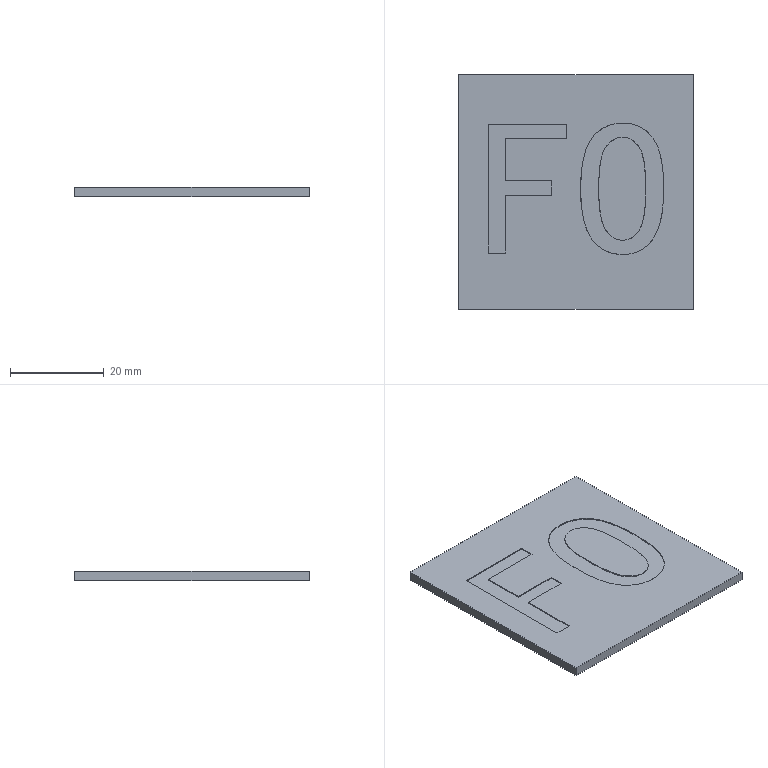Part | STEP file | lll_id1630_x_t | 1 solid | 22 faces | box 50 x 50 x 2 mm | volume 4919 mm3 | plane 19 | other 3
STEP:
#1=CARTESIAN_POINT('',(2722.277,-531.694,3.259));
#2=VERTEX_POINT('',#1);
#3=CARTESIAN_POINT('',(2739.088,-531.694,3.259));
#4=VERTEX_POINT('',#3);
#5=CARTESIAN_POINT('',(2730.683,-531.694,3.259));
#6=DIRECTION('',(1.,0.,0.));
#7=VECTOR('',#6,1.);
#8=LINE('',#5,#7);
#9=EDGE_CURVE('',#2,#4,#8,.T.);
#10=ORIENTED_EDGE('',*,*,#9,.T.);
#11=CARTESIAN_POINT('',(2739.088,-534.734,3.259));
#12=VERTEX_POINT('',#11);
#13=CARTESIAN_POINT('',(2739.088,-533.214,3.259));
#14=DIRECTION('',(0.,-1.,0.));
#15=VECTOR('',#14,1.);
#16=LINE('',#13,#15);
#17=EDGE_CURVE('',#4,#12,#16,.T.);
#18=ORIENTED_EDGE('',*,*,#17,.T.);
#19=CARTESIAN_POINT('',(2725.962,-534.734,3.259));
#20=VERTEX_POINT('',#19);
#21=CARTESIAN_POINT('',(2732.525,-534.734,3.259));
#22=DIRECTION('',(-1.,0.,0.));
#23=VECTOR('',#22,1.);
#24=LINE('',#21,#23);
#25=EDGE_CURVE('',#12,#20,#24,.T.);
#26=ORIENTED_EDGE('',*,*,#25,.T.);
#27=CARTESIAN_POINT('',(2725.962,-543.702,3.259));
#28=VERTEX_POINT('',#27);
#29=CARTESIAN_POINT('',(2725.962,-539.218,3.259));
#30=DIRECTION('',(0.,-1.,0.));
#31=VECTOR('',#30,1.);
#32=LINE('',#29,#31);
#33=EDGE_CURVE('',#20,#28,#32,.T.);
#34=ORIENTED_EDGE('',*,*,#33,.T.);
#35=CARTESIAN_POINT('',(2735.884,-543.702,3.259));
#36=VERTEX_POINT('',#35);
#37=CARTESIAN_POINT('',(2730.923,-543.702,3.259));
#38=DIRECTION('',(1.,0.,0.));
#39=VECTOR('',#38,1.);
#40=LINE('',#37,#39);
#41=EDGE_CURVE('',#28,#36,#40,.T.);
#42=ORIENTED_EDGE('',*,*,#41,.T.);
#43=CARTESIAN_POINT('',(2735.884,-546.742,3.259));
#44=VERTEX_POINT('',#43);
#45=CARTESIAN_POINT('',(2735.884,-545.222,3.259));
#46=DIRECTION('',(0.,-1.,0.));
#47=VECTOR('',#46,1.);
#48=LINE('',#45,#47);
#49=EDGE_CURVE('',#36,#44,#48,.T.);
#50=ORIENTED_EDGE('',*,*,#49,.T.);
#51=CARTESIAN_POINT('',(2725.962,-546.742,3.259));
#52=VERTEX_POINT('',#51);
#53=CARTESIAN_POINT('',(2730.923,-546.742,3.259));
#54=DIRECTION('',(-1.,0.,0.));
#55=VECTOR('',#54,1.);
#56=LINE('',#53,#55);
#57=EDGE_CURVE('',#44,#52,#56,.T.);
#58=ORIENTED_EDGE('',*,*,#57,.T.);
#59=CARTESIAN_POINT('',(2725.962,-559.065,3.259));
#60=VERTEX_POINT('',#59);
#61=CARTESIAN_POINT('',(2725.962,-552.903,3.259));
#62=DIRECTION('',(0.,-1.,0.));
#63=VECTOR('',#62,1.);
#64=LINE('',#61,#63);
#65=EDGE_CURVE('',#52,#60,#64,.T.);
#66=ORIENTED_EDGE('',*,*,#65,.T.);
#67=CARTESIAN_POINT('',(2722.277,-559.065,3.259));
#68=VERTEX_POINT('',#67);
#69=CARTESIAN_POINT('',(2724.119,-559.065,3.259));
#70=DIRECTION('',(-1.,0.,0.));
#71=VECTOR('',#70,1.);
#72=LINE('',#69,#71);
#73=EDGE_CURVE('',#60,#68,#72,.T.);
#74=ORIENTED_EDGE('',*,*,#73,.T.);
#75=CARTESIAN_POINT('',(2722.277,-545.38,3.259));
#76=DIRECTION('',(0.,1.,0.));
#77=VECTOR('',#76,1.);
#78=LINE('',#75,#77);
#79=EDGE_CURVE('',#68,#2,#78,.T.);
#80=ORIENTED_EDGE('',*,*,#79,.T.);
#81=EDGE_LOOP('',(#10,#18,#26,#34,#42,#50,#58,#66,#74,#80));
#82=FACE_BOUND('',#81,.T.);
#83=CARTESIAN_POINT('',(2766.009,-571.065,3.259));
#84=VERTEX_POINT('',#83);
#85=CARTESIAN_POINT('',(2716.009,-571.065,3.259));
#86=VERTEX_POINT('',#85);
#87=CARTESIAN_POINT('',(2816.009,-571.065,3.259));
#88=DIRECTION('',(-1.,0.,0.));
#89=VECTOR('',#88,1.);
#90=LINE('',#87,#89);
#91=EDGE_CURVE('',#84,#86,#90,.T.);
#92=ORIENTED_EDGE('',*,*,#91,.F.);
#93=CARTESIAN_POINT('',(2766.009,-521.065,3.259));
#94=VERTEX_POINT('',#93);
#95=CARTESIAN_POINT('',(2766.009,-471.065,3.259));
#96=DIRECTION('',(0.,-1.,0.));
#97=VECTOR('',#96,1.);
#98=LINE('',#95,#97);
#99=EDGE_CURVE('',#94,#84,#98,.T.);
#100=ORIENTED_EDGE('',*,*,#99,.F.);
#101=CARTESIAN_POINT('',(2716.009,-521.065,3.259));
#102=VERTEX_POINT('',#101);
#103=CARTESIAN_POINT('',(2816.009,-521.065,3.259));
#104=DIRECTION('',(-1.,0.,0.));
#105=VECTOR('',#104,1.);
#106=LINE('',#103,#105);
#107=EDGE_CURVE('',#94,#102,#106,.T.);
#108=ORIENTED_EDGE('',*,*,#107,.T.);
#109=CARTESIAN_POINT('',(2716.009,-471.065,3.259));
#110=DIRECTION('',(0.,1.,0.));
#111=VECTOR('',#110,1.);
#112=LINE('',#109,#111);
#113=EDGE_CURVE('',#86,#102,#112,.T.);
#114=ORIENTED_EDGE('',*,*,#113,.F.);
#115=EDGE_LOOP('',(#92,#100,#108,#114));
#116=FACE_BOUND('',#115,.T.);
#117=CARTESIAN_POINT('',(2744.372,-556.108,3.259));
#118=VERTEX_POINT('',#117);
#119=CARTESIAN_POINT('',(2757.423,-534.576,3.259));
#120=VERTEX_POINT('',#119);
#121=CARTESIAN_POINT('',(2744.372,-556.108,3.259));
#122=CARTESIAN_POINT('',(2742.765,-553.923,3.259));
#123=CARTESIAN_POINT('',(2741.97,-550.314,3.259));
#124=CARTESIAN_POINT('',(2741.97,-540.28,3.259));
#125=CARTESIAN_POINT('',(2742.773,-536.707,3.259));
#126=CARTESIAN_POINT('',(2745.977,-532.436,3.259));
#127=CARTESIAN_POINT('',(2748.162,-531.371,3.259));
#128=CARTESIAN_POINT('',(2753.715,-531.371,3.259));
#129=CARTESIAN_POINT('',(2755.877,-532.437,3.259));
#130=CARTESIAN_POINT('',(2757.423,-534.576,3.259));
#131=B_SPLINE_CURVE_WITH_KNOTS('',3,(#121,#122,#123,#124,#125,#126,#127,#128,#129,#130),.UNSPECIFIED.,.F.,.F.,(4,2,2,2,4),(0.,0.2492,0.4988,0.7494,1.),.UNSPECIFIED.);
#132=EDGE_CURVE('',#118,#120,#131,.T.);
#133=ORIENTED_EDGE('',*,*,#132,.T.);
#134=CARTESIAN_POINT('',(2757.423,-534.576,3.259));
#135=CARTESIAN_POINT('',(2758.969,-536.707,3.259));
#136=CARTESIAN_POINT('',(2759.742,-540.28,3.259));
#137=CARTESIAN_POINT('',(2759.742,-550.314,3.259));
#138=CARTESIAN_POINT('',(2758.969,-553.917,3.259));
#139=CARTESIAN_POINT('',(2755.88,-558.294,3.259));
#140=CARTESIAN_POINT('',(2753.715,-559.388,3.259));
#141=CARTESIAN_POINT('',(2748.162,-559.388,3.259));
#142=CARTESIAN_POINT('',(2745.978,-558.292,3.259));
#143=CARTESIAN_POINT('',(2744.372,-556.108,3.259));
#144=B_SPLINE_CURVE_WITH_KNOTS('',3,(#134,#135,#136,#137,#138,#139,#140,#141,#142,#143),.UNSPECIFIED.,.F.,.F.,(4,2,2,2,4),(0.,0.2506,0.5008,0.7504,1.),.UNSPECIFIED.);
#145=EDGE_CURVE('',#120,#118,#144,.T.);
#146=ORIENTED_EDGE('',*,*,#145,.T.);
#147=EDGE_LOOP('',(#133,#146));
#148=FACE_BOUND('',#147,.T.);
#149=CARTESIAN_POINT('',(2816.009,-471.065,3.259));
#150=DIRECTION('',(0.,0.,1.));
#151=DIRECTION('',(1.,0.,0.));
#152=AXIS2_PLACEMENT_3D('',#149,#150,#151);
#153=PLANE('',#152);
#154=ADVANCED_FACE('',(#82,#116,#148),#153,.T.);
#155=CARTESIAN_POINT('',(2766.009,-571.065,1.259));
#156=VERTEX_POINT('',#155);
#157=CARTESIAN_POINT('',(2766.009,-571.065,179.534));
#158=DIRECTION('',(0.,0.,1.));
#159=VECTOR('',#158,1.);
#160=LINE('',#157,#159);
#161=EDGE_CURVE('',#156,#84,#160,.T.);
#162=ORIENTED_EDGE('',*,*,#161,.F.);
#163=CARTESIAN_POINT('',(2766.009,-521.065,1.259));
#164=VERTEX_POINT('',#163);
#165=CARTESIAN_POINT('',(2766.009,-471.065,1.259));
#166=DIRECTION('',(0.,-1.,0.));
#167=VECTOR('',#166,1.);
#168=LINE('',#165,#167);
#169=EDGE_CURVE('',#164,#156,#168,.T.);
#170=ORIENTED_EDGE('',*,*,#169,.F.);
#171=CARTESIAN_POINT('',(2766.009,-521.065,2.109));
#172=DIRECTION('',(0.,0.,-1.));
#173=VECTOR('',#172,1.);
#174=LINE('',#171,#173);
#175=EDGE_CURVE('',#94,#164,#174,.T.);
#176=ORIENTED_EDGE('',*,*,#175,.F.);
#177=ORIENTED_EDGE('',*,*,#99,.T.);
#178=EDGE_LOOP('',(#162,#170,#176,#177));
#179=FACE_OUTER_BOUND('',#178,.T.);
#180=CARTESIAN_POINT('',(2766.009,-546.065,2.259));
#181=DIRECTION('',(1.,0.,0.));
#182=DIRECTION('',(0.,0.,-1.));
#183=AXIS2_PLACEMENT_3D('',#180,#181,#182);
#184=PLANE('',#183);
#185=ADVANCED_FACE('',(#179),#184,.T.);
#186=CARTESIAN_POINT('',(2716.009,-521.065,1.259));
#187=VERTEX_POINT('',#186);
#188=CARTESIAN_POINT('',(2716.009,-521.065,2.109));
#189=DIRECTION('',(0.,0.,1.));
#190=VECTOR('',#189,1.);
#191=LINE('',#188,#190);
#192=EDGE_CURVE('',#187,#102,#191,.T.);
#193=ORIENTED_EDGE('',*,*,#192,.F.);
#194=CARTESIAN_POINT('',(2716.009,-571.065,1.259));
#195=VERTEX_POINT('',#194);
#196=CARTESIAN_POINT('',(2716.009,-471.065,1.259));
#197=DIRECTION('',(0.,-1.,0.));
#198=VECTOR('',#197,1.);
#199=LINE('',#196,#198);
#200=EDGE_CURVE('',#187,#195,#199,.T.);
#201=ORIENTED_EDGE('',*,*,#200,.T.);
#202=CARTESIAN_POINT('',(2716.009,-571.065,179.534));
#203=DIRECTION('',(0.,0.,1.));
#204=VECTOR('',#203,1.);
#205=LINE('',#202,#204);
#206=EDGE_CURVE('',#195,#86,#205,.T.);
#207=ORIENTED_EDGE('',*,*,#206,.T.);
#208=ORIENTED_EDGE('',*,*,#113,.T.);
#209=EDGE_LOOP('',(#193,#201,#207,#208));
#210=FACE_OUTER_BOUND('',#209,.T.);
#211=CARTESIAN_POINT('',(2716.009,-521.065,2.109));
#212=DIRECTION('',(1.,0.,0.));
#213=DIRECTION('',(0.,0.,-1.));
#214=AXIS2_PLACEMENT_3D('',#211,#212,#213);
#215=PLANE('',#214);
#216=ADVANCED_FACE('',(#210),#215,.F.);
#217=ORIENTED_EDGE('',*,*,#107,.F.);
#218=ORIENTED_EDGE('',*,*,#175,.T.);
#219=CARTESIAN_POINT('',(1256.009,-521.065,1.259));
#220=DIRECTION('',(1.,0.,0.));
#221=VECTOR('',#220,1.);
#222=LINE('',#219,#221);
#223=EDGE_CURVE('',#187,#164,#222,.T.);
#224=ORIENTED_EDGE('',*,*,#223,.F.);
#225=ORIENTED_EDGE('',*,*,#192,.T.);
#226=EDGE_LOOP('',(#217,#218,#224,#225));
#227=FACE_OUTER_BOUND('',#226,.T.);
#228=CARTESIAN_POINT('',(2766.009,-521.065,2.109));
#229=DIRECTION('',(0.,1.,0.));
#230=DIRECTION('',(0.,0.,1.));
#231=AXIS2_PLACEMENT_3D('',#228,#229,#230);
#232=PLANE('',#231);
#233=ADVANCED_FACE('',(#227),#232,.T.);
#234=CARTESIAN_POINT('',(-4500.12,-571.065,1.259));
#235=DIRECTION('',(1.,0.,0.));
#236=VECTOR('',#235,1.);
#237=LINE('',#234,#236);
#238=EDGE_CURVE('',#195,#156,#237,.T.);
#239=ORIENTED_EDGE('',*,*,#238,.T.);
#240=ORIENTED_EDGE('',*,*,#161,.T.);
#241=ORIENTED_EDGE('',*,*,#91,.T.);
#242=ORIENTED_EDGE('',*,*,#206,.F.);
#243=EDGE_LOOP('',(#239,#240,#241,#242));
#244=FACE_OUTER_BOUND('',#243,.T.);
#245=CARTESIAN_POINT('',(-4500.12,-571.065,179.534));
#246=DIRECTION('',(0.,-1.,0.));
#247=DIRECTION('',(0.,0.,-1.));
#248=AXIS2_PLACEMENT_3D('',#245,#246,#247);
#249=PLANE('',#248);
#250=ADVANCED_FACE('',(#244),#249,.T.);
#251=ORIENTED_EDGE('',*,*,#223,.T.);
#252=ORIENTED_EDGE('',*,*,#169,.T.);
#253=ORIENTED_EDGE('',*,*,#238,.F.);
#254=ORIENTED_EDGE('',*,*,#200,.F.);
#255=EDGE_LOOP('',(#251,#252,#253,#254));
#256=FACE_OUTER_BOUND('',#255,.T.);
#257=CARTESIAN_POINT('',(1256.009,-471.065,1.259));
#258=DIRECTION('',(0.,0.,-1.));
#259=DIRECTION('',(-1.,0.,0.));
#260=AXIS2_PLACEMENT_3D('',#257,#258,#259);
#261=PLANE('',#260);
#262=ADVANCED_FACE('',(#256),#261,.T.);
#263=ORIENTED_EDGE('',*,*,#17,.F.);
#264=CARTESIAN_POINT('',(2739.088,-531.694,3.059));
#265=VERTEX_POINT('',#264);
#266=CARTESIAN_POINT('',(2739.088,-531.694,3.059));
#267=DIRECTION('',(0.,0.,-1.));
#268=VECTOR('',#267,1.);
#269=LINE('',#266,#268);
#270=EDGE_CURVE('',#4,#265,#269,.T.);
#271=ORIENTED_EDGE('',*,*,#270,.T.);
#272=CARTESIAN_POINT('',(2739.088,-534.734,3.059));
#273=VERTEX_POINT('',#272);
#274=CARTESIAN_POINT('',(2739.088,-533.214,3.059));
#275=DIRECTION('',(0.,1.,0.));
#276=VECTOR('',#275,1.);
#277=LINE('',#274,#276);
#278=EDGE_CURVE('',#273,#265,#277,.T.);
#279=ORIENTED_EDGE('',*,*,#278,.F.);
#280=CARTESIAN_POINT('',(2739.088,-534.734,3.059));
#281=DIRECTION('',(0.,0.,-1.));
#282=VECTOR('',#281,1.);
#283=LINE('',#280,#282);
#284=EDGE_CURVE('',#12,#273,#283,.T.);
#285=ORIENTED_EDGE('',*,*,#284,.F.);
#286=EDGE_LOOP('',(#263,#271,#279,#285));
#287=FACE_OUTER_BOUND('',#286,.T.);
#288=CARTESIAN_POINT('',(2739.088,-531.694,3.059));
#289=DIRECTION('',(-1.,0.,0.));
#290=DIRECTION('',(0.,0.,1.));
#291=AXIS2_PLACEMENT_3D('',#288,#289,#290);
#292=PLANE('',#291);
#293=ADVANCED_FACE('',(#287),#292,.T.);
#294=ORIENTED_EDGE('',*,*,#25,.F.);
#295=ORIENTED_EDGE('',*,*,#284,.T.);
#296=CARTESIAN_POINT('',(2725.962,-534.734,3.059));
#297=VERTEX_POINT('',#296);
#298=CARTESIAN_POINT('',(2732.525,-534.734,3.059));
#299=DIRECTION('',(1.,0.,0.));
#300=VECTOR('',#299,1.);
#301=LINE('',#298,#300);
#302=EDGE_CURVE('',#297,#273,#301,.T.);
#303=ORIENTED_EDGE('',*,*,#302,.F.);
#304=CARTESIAN_POINT('',(2725.962,-534.734,3.059));
#305=DIRECTION('',(0.,0.,-1.));
#306=VECTOR('',#305,1.);
#307=LINE('',#304,#306);
#308=EDGE_CURVE('',#20,#297,#307,.T.);
#309=ORIENTED_EDGE('',*,*,#308,.F.);
#310=EDGE_LOOP('',(#294,#295,#303,#309));
#311=FACE_OUTER_BOUND('',#310,.T.);
#312=CARTESIAN_POINT('',(2739.088,-534.734,3.059));
#313=DIRECTION('',(0.,1.,0.));
#314=DIRECTION('',(0.,0.,1.));
#315=AXIS2_PLACEMENT_3D('',#312,#313,#314);
#316=PLANE('',#315);
#317=ADVANCED_FACE('',(#311),#316,.T.);
#318=ORIENTED_EDGE('',*,*,#33,.F.);
#319=ORIENTED_EDGE('',*,*,#308,.T.);
#320=CARTESIAN_POINT('',(2725.962,-543.702,3.059));
#321=VERTEX_POINT('',#320);
#322=CARTESIAN_POINT('',(2725.962,-539.218,3.059));
#323=DIRECTION('',(0.,1.,0.));
#324=VECTOR('',#323,1.);
#325=LINE('',#322,#324);
#326=EDGE_CURVE('',#321,#297,#325,.T.);
#327=ORIENTED_EDGE('',*,*,#326,.F.);
#328=CARTESIAN_POINT('',(2725.962,-543.702,3.059));
#329=DIRECTION('',(0.,0.,-1.));
#330=VECTOR('',#329,1.);
#331=LINE('',#328,#330);
#332=EDGE_CURVE('',#28,#321,#331,.T.);
#333=ORIENTED_EDGE('',*,*,#332,.F.);
#334=EDGE_LOOP('',(#318,#319,#327,#333));
#335=FACE_OUTER_BOUND('',#334,.T.);
#336=CARTESIAN_POINT('',(2725.962,-534.734,3.059));
#337=DIRECTION('',(-1.,0.,0.));
#338=DIRECTION('',(0.,0.,1.));
#339=AXIS2_PLACEMENT_3D('',#336,#337,#338);
#340=PLANE('',#339);
#341=ADVANCED_FACE('',(#335),#340,.T.);
#342=ORIENTED_EDGE('',*,*,#41,.F.);
#343=ORIENTED_EDGE('',*,*,#332,.T.);
#344=CARTESIAN_POINT('',(2735.884,-543.702,3.059));
#345=VERTEX_POINT('',#344);
#346=CARTESIAN_POINT('',(2730.923,-543.702,3.059));
#347=DIRECTION('',(-1.,0.,0.));
#348=VECTOR('',#347,1.);
#349=LINE('',#346,#348);
#350=EDGE_CURVE('',#345,#321,#349,.T.);
#351=ORIENTED_EDGE('',*,*,#350,.F.);
#352=CARTESIAN_POINT('',(2735.884,-543.702,3.059));
#353=DIRECTION('',(0.,0.,-1.));
#354=VECTOR('',#353,1.);
#355=LINE('',#352,#354);
#356=EDGE_CURVE('',#36,#345,#355,.T.);
#357=ORIENTED_EDGE('',*,*,#356,.F.);
#358=EDGE_LOOP('',(#342,#343,#351,#357));
#359=FACE_OUTER_BOUND('',#358,.T.);
#360=CARTESIAN_POINT('',(2725.962,-543.702,3.059));
#361=DIRECTION('',(0.,-1.,0.));
#362=DIRECTION('',(0.,0.,-1.));
#363=AXIS2_PLACEMENT_3D('',#360,#361,#362);
#364=PLANE('',#363);
#365=ADVANCED_FACE('',(#359),#364,.T.);
#366=ORIENTED_EDGE('',*,*,#49,.F.);
#367=ORIENTED_EDGE('',*,*,#356,.T.);
#368=CARTESIAN_POINT('',(2735.884,-546.742,3.059));
#369=VERTEX_POINT('',#368);
#370=CARTESIAN_POINT('',(2735.884,-545.222,3.059));
#371=DIRECTION('',(0.,1.,0.));
#372=VECTOR('',#371,1.);
#373=LINE('',#370,#372);
#374=EDGE_CURVE('',#369,#345,#373,.T.);
#375=ORIENTED_EDGE('',*,*,#374,.F.);
#376=CARTESIAN_POINT('',(2735.884,-546.742,3.059));
#377=DIRECTION('',(0.,0.,-1.));
#378=VECTOR('',#377,1.);
#379=LINE('',#376,#378);
#380=EDGE_CURVE('',#44,#369,#379,.T.);
#381=ORIENTED_EDGE('',*,*,#380,.F.);
#382=EDGE_LOOP('',(#366,#367,#375,#381));
#383=FACE_OUTER_BOUND('',#382,.T.);
#384=CARTESIAN_POINT('',(2735.884,-543.702,3.059));
#385=DIRECTION('',(-1.,0.,0.));
#386=DIRECTION('',(0.,0.,1.));
#387=AXIS2_PLACEMENT_3D('',#384,#385,#386);
#388=PLANE('',#387);
#389=ADVANCED_FACE('',(#383),#388,.T.);
#390=ORIENTED_EDGE('',*,*,#57,.F.);
#391=ORIENTED_EDGE('',*,*,#380,.T.);
#392=CARTESIAN_POINT('',(2725.962,-546.742,3.059));
#393=VERTEX_POINT('',#392);
#394=CARTESIAN_POINT('',(2730.923,-546.742,3.059));
#395=DIRECTION('',(1.,0.,0.));
#396=VECTOR('',#395,1.);
#397=LINE('',#394,#396);
#398=EDGE_CURVE('',#393,#369,#397,.T.);
#399=ORIENTED_EDGE('',*,*,#398,.F.);
#400=CARTESIAN_POINT('',(2725.962,-546.742,3.059));
#401=DIRECTION('',(0.,0.,-1.));
#402=VECTOR('',#401,1.);
#403=LINE('',#400,#402);
#404=EDGE_CURVE('',#52,#393,#403,.T.);
#405=ORIENTED_EDGE('',*,*,#404,.F.);
#406=EDGE_LOOP('',(#390,#391,#399,#405));
#407=FACE_OUTER_BOUND('',#406,.T.);
#408=CARTESIAN_POINT('',(2735.884,-546.742,3.059));
#409=DIRECTION('',(0.,1.,0.));
#410=DIRECTION('',(0.,0.,1.));
#411=AXIS2_PLACEMENT_3D('',#408,#409,#410);
#412=PLANE('',#411);
#413=ADVANCED_FACE('',(#407),#412,.T.);
#414=ORIENTED_EDGE('',*,*,#65,.F.);
#415=ORIENTED_EDGE('',*,*,#404,.T.);
#416=CARTESIAN_POINT('',(2725.962,-559.065,3.059));
#417=VERTEX_POINT('',#416);
#418=CARTESIAN_POINT('',(2725.962,-552.903,3.059));
#419=DIRECTION('',(0.,1.,0.));
#420=VECTOR('',#419,1.);
#421=LINE('',#418,#420);
#422=EDGE_CURVE('',#417,#393,#421,.T.);
#423=ORIENTED_EDGE('',*,*,#422,.F.);
#424=CARTESIAN_POINT('',(2725.962,-559.065,3.059));
#425=DIRECTION('',(0.,0.,-1.));
#426=VECTOR('',#425,1.);
#427=LINE('',#424,#426);
#428=EDGE_CURVE('',#60,#417,#427,.T.);
#429=ORIENTED_EDGE('',*,*,#428,.F.);
#430=EDGE_LOOP('',(#414,#415,#423,#429));
#431=FACE_OUTER_BOUND('',#430,.T.);
#432=CARTESIAN_POINT('',(2725.962,-546.742,3.059));
#433=DIRECTION('',(-1.,0.,0.));
#434=DIRECTION('',(0.,0.,1.));
#435=AXIS2_PLACEMENT_3D('',#432,#433,#434);
#436=PLANE('',#435);
#437=ADVANCED_FACE('',(#431),#436,.T.);
#438=ORIENTED_EDGE('',*,*,#73,.F.);
#439=ORIENTED_EDGE('',*,*,#428,.T.);
#440=CARTESIAN_POINT('',(2722.277,-559.065,3.059));
#441=VERTEX_POINT('',#440);
#442=CARTESIAN_POINT('',(2724.119,-559.065,3.059));
#443=DIRECTION('',(1.,0.,0.));
#444=VECTOR('',#443,1.);
#445=LINE('',#442,#444);
#446=EDGE_CURVE('',#441,#417,#445,.T.);
#447=ORIENTED_EDGE('',*,*,#446,.F.);
#448=CARTESIAN_POINT('',(2722.277,-559.065,3.059));
#449=DIRECTION('',(0.,0.,-1.));
#450=VECTOR('',#449,1.);
#451=LINE('',#448,#450);
#452=EDGE_CURVE('',#68,#441,#451,.T.);
#453=ORIENTED_EDGE('',*,*,#452,.F.);
#454=EDGE_LOOP('',(#438,#439,#447,#453));
#455=FACE_OUTER_BOUND('',#454,.T.);
#456=CARTESIAN_POINT('',(2725.962,-559.065,3.059));
#457=DIRECTION('',(0.,1.,0.));
#458=DIRECTION('',(0.,0.,1.));
#459=AXIS2_PLACEMENT_3D('',#456,#457,#458);
#460=PLANE('',#459);
#461=ADVANCED_FACE('',(#455),#460,.T.);
#462=ORIENTED_EDGE('',*,*,#79,.F.);
#463=ORIENTED_EDGE('',*,*,#452,.T.);
#464=CARTESIAN_POINT('',(2722.277,-531.694,3.059));
#465=VERTEX_POINT('',#464);
#466=CARTESIAN_POINT('',(2722.277,-545.38,3.059));
#467=DIRECTION('',(0.,-1.,0.));
#468=VECTOR('',#467,1.);
#469=LINE('',#466,#468);
#470=EDGE_CURVE('',#465,#441,#469,.T.);
#471=ORIENTED_EDGE('',*,*,#470,.F.);
#472=CARTESIAN_POINT('',(2722.277,-531.694,3.059));
#473=DIRECTION('',(0.,0.,-1.));
#474=VECTOR('',#473,1.);
#475=LINE('',#472,#474);
#476=EDGE_CURVE('',#2,#465,#475,.T.);
#477=ORIENTED_EDGE('',*,*,#476,.F.);
#478=EDGE_LOOP('',(#462,#463,#471,#477));
#479=FACE_OUTER_BOUND('',#478,.T.);
#480=CARTESIAN_POINT('',(2722.277,-559.065,3.059));
#481=DIRECTION('',(1.,0.,0.));
#482=DIRECTION('',(0.,0.,-1.));
#483=AXIS2_PLACEMENT_3D('',#480,#481,#482);
#484=PLANE('',#483);
#485=ADVANCED_FACE('',(#479),#484,.T.);
#486=ORIENTED_EDGE('',*,*,#9,.F.);
#487=ORIENTED_EDGE('',*,*,#476,.T.);
#488=CARTESIAN_POINT('',(2730.683,-531.694,3.059));
#489=DIRECTION('',(-1.,0.,0.));
#490=VECTOR('',#489,1.);
#491=LINE('',#488,#490);
#492=EDGE_CURVE('',#265,#465,#491,.T.);
#493=ORIENTED_EDGE('',*,*,#492,.F.);
#494=ORIENTED_EDGE('',*,*,#270,.F.);
#495=EDGE_LOOP('',(#486,#487,#493,#494));
#496=FACE_OUTER_BOUND('',#495,.T.);
#497=CARTESIAN_POINT('',(2722.277,-531.694,3.059));
#498=DIRECTION('',(0.,-1.,0.));
#499=DIRECTION('',(0.,0.,-1.));
#500=AXIS2_PLACEMENT_3D('',#497,#498,#499);
#501=PLANE('',#500);
#502=ADVANCED_FACE('',(#496),#501,.T.);
#503=ORIENTED_EDGE('',*,*,#278,.T.);
#504=ORIENTED_EDGE('',*,*,#492,.T.);
#505=ORIENTED_EDGE('',*,*,#470,.T.);
#506=ORIENTED_EDGE('',*,*,#446,.T.);
#507=ORIENTED_EDGE('',*,*,#422,.T.);
#508=ORIENTED_EDGE('',*,*,#398,.T.);
#509=ORIENTED_EDGE('',*,*,#374,.T.);
#510=ORIENTED_EDGE('',*,*,#350,.T.);
#511=ORIENTED_EDGE('',*,*,#326,.T.);
#512=ORIENTED_EDGE('',*,*,#302,.T.);
#513=EDGE_LOOP('',(#503,#504,#505,#506,#507,#508,#509,#510,#511,#512));
#514=FACE_OUTER_BOUND('',#513,.T.);
#515=CARTESIAN_POINT('',(2739.088,-533.214,3.059));
#516=DIRECTION('',(0.,0.,1.));
#517=DIRECTION('',(1.,0.,0.));
#518=AXIS2_PLACEMENT_3D('',#515,#516,#517);
#519=PLANE('',#518);
#520=ADVANCED_FACE('',(#514),#519,.T.);
#521=ORIENTED_EDGE('',*,*,#145,.F.);
#522=CARTESIAN_POINT('',(2757.423,-534.576,3.059));
#523=VERTEX_POINT('',#522);
#524=CARTESIAN_POINT('',(2757.423,-534.576,3.059));
#525=DIRECTION('',(0.,0.,1.));
#526=VECTOR('',#525,1.);
#527=LINE('',#524,#526);
#528=EDGE_CURVE('',#523,#120,#527,.T.);
#529=ORIENTED_EDGE('',*,*,#528,.F.);
#530=CARTESIAN_POINT('',(2744.372,-556.108,3.059));
#531=VERTEX_POINT('',#530);
#532=CARTESIAN_POINT('',(2744.372,-556.108,3.059));
#533=CARTESIAN_POINT('',(2745.978,-558.292,3.059));
#534=CARTESIAN_POINT('',(2748.162,-559.388,3.059));
#535=CARTESIAN_POINT('',(2753.715,-559.388,3.059));
#536=CARTESIAN_POINT('',(2755.88,-558.294,3.059));
#537=CARTESIAN_POINT('',(2758.969,-553.917,3.059));
#538=CARTESIAN_POINT('',(2759.742,-550.314,3.059));
#539=CARTESIAN_POINT('',(2759.742,-540.28,3.059));
#540=CARTESIAN_POINT('',(2758.969,-536.707,3.059));
#541=CARTESIAN_POINT('',(2757.423,-534.576,3.059));
#542=B_SPLINE_CURVE_WITH_KNOTS('',3,(#532,#533,#534,#535,#536,#537,#538,#539,#540,#541),.UNSPECIFIED.,.F.,.F.,(4,2,2,2,4),(0.,0.2496,0.4992,0.7494,1.),.UNSPECIFIED.);
#543=EDGE_CURVE('',#531,#523,#542,.T.);
#544=ORIENTED_EDGE('',*,*,#543,.F.);
#545=CARTESIAN_POINT('',(2744.372,-556.108,3.059));
#546=DIRECTION('',(0.,0.,-1.));
#547=VECTOR('',#546,1.);
#548=LINE('',#545,#547);
#549=EDGE_CURVE('',#118,#531,#548,.T.);
#550=ORIENTED_EDGE('',*,*,#549,.F.);
#551=EDGE_LOOP('',(#521,#529,#544,#550));
#552=FACE_OUTER_BOUND('',#551,.T.);
#553=CARTESIAN_POINT('',(2757.423,-534.576,3.059));
#554=CARTESIAN_POINT('',(2758.969,-536.707,3.059));
#555=CARTESIAN_POINT('',(2759.742,-540.28,3.059));
#556=CARTESIAN_POINT('',(2759.742,-550.314,3.059));
#557=CARTESIAN_POINT('',(2758.969,-553.917,3.059));
#558=CARTESIAN_POINT('',(2755.88,-558.294,3.059));
#559=CARTESIAN_POINT('',(2753.715,-559.388,3.059));
#560=CARTESIAN_POINT('',(2748.162,-559.388,3.059));
#561=CARTESIAN_POINT('',(2745.978,-558.292,3.059));
#562=CARTESIAN_POINT('',(2744.372,-556.108,3.059));
#563=B_SPLINE_CURVE_WITH_KNOTS('',3,(#553,#554,#555,#556,#557,#558,#559,#560,#561,#562),.UNSPECIFIED.,.F.,.F.,(4,2,2,2,4),(0.,0.2506,0.5008,0.7504,1.),.UNSPECIFIED.);
#564=DIRECTION('',(0.,0.,1.));
#565=VECTOR('',#564,1.);
#566=SURFACE_OF_LINEAR_EXTRUSION('',#563,#565);
#567=ADVANCED_FACE('',(#552),#566,.T.);
#568=ORIENTED_EDGE('',*,*,#132,.F.);
#569=ORIENTED_EDGE('',*,*,#549,.T.);
#570=CARTESIAN_POINT('',(2757.423,-534.576,3.059));
#571=CARTESIAN_POINT('',(2755.877,-532.437,3.059));
#572=CARTESIAN_POINT('',(2753.715,-531.371,3.059));
#573=CARTESIAN_POINT('',(2748.162,-531.371,3.059));
#574=CARTESIAN_POINT('',(2745.977,-532.436,3.059));
#575=CARTESIAN_POINT('',(2742.773,-536.707,3.059));
#576=CARTESIAN_POINT('',(2741.97,-540.28,3.059));
#577=CARTESIAN_POINT('',(2741.97,-550.314,3.059));
#578=CARTESIAN_POINT('',(2742.765,-553.923,3.059));
#579=CARTESIAN_POINT('',(2744.372,-556.108,3.059));
#580=B_SPLINE_CURVE_WITH_KNOTS('',3,(#570,#571,#572,#573,#574,#575,#576,#577,#578,#579),.UNSPECIFIED.,.F.,.F.,(4,2,2,2,4),(0.,0.2506,0.5012,0.7508,1.),.UNSPECIFIED.);
#581=EDGE_CURVE('',#523,#531,#580,.T.);
#582=ORIENTED_EDGE('',*,*,#581,.F.);
#583=ORIENTED_EDGE('',*,*,#528,.T.);
#584=EDGE_LOOP('',(#568,#569,#582,#583));
#585=FACE_OUTER_BOUND('',#584,.T.);
#586=CARTESIAN_POINT('',(2744.372,-556.108,3.059));
#587=CARTESIAN_POINT('',(2742.765,-553.923,3.059));
#588=CARTESIAN_POINT('',(2741.97,-550.314,3.059));
#589=CARTESIAN_POINT('',(2741.97,-540.28,3.059));
#590=CARTESIAN_POINT('',(2742.773,-536.707,3.059));
#591=CARTESIAN_POINT('',(2745.977,-532.436,3.059));
#592=CARTESIAN_POINT('',(2748.162,-531.371,3.059));
#593=CARTESIAN_POINT('',(2753.715,-531.371,3.059));
#594=CARTESIAN_POINT('',(2755.877,-532.437,3.059));
#595=CARTESIAN_POINT('',(2757.423,-534.576,3.059));
#596=B_SPLINE_CURVE_WITH_KNOTS('',3,(#586,#587,#588,#589,#590,#591,#592,#593,#594,#595),.UNSPECIFIED.,.F.,.F.,(4,2,2,2,4),(0.,0.2492,0.4988,0.7494,1.),.UNSPECIFIED.);
#597=DIRECTION('',(0.,0.,1.));
#598=VECTOR('',#597,1.);
#599=SURFACE_OF_LINEAR_EXTRUSION('',#596,#598);
#600=ADVANCED_FACE('',(#585),#599,.T.);
#601=CARTESIAN_POINT('',(2754.458,-554.187,3.059));
#602=VERTEX_POINT('',#601);
#603=CARTESIAN_POINT('',(2755.419,-552.746,3.059));
#604=CARTESIAN_POINT('',(2753.498,-555.628,3.059));
#605=CARTESIAN_POINT('',(2752.327,-556.348,3.059));
#606=CARTESIAN_POINT('',(2749.55,-556.348,3.059));
#607=CARTESIAN_POINT('',(2748.349,-555.628,3.059));
#608=CARTESIAN_POINT('',(2746.323,-552.746,3.059));
#609=CARTESIAN_POINT('',(2745.813,-549.781,3.059));
#610=CARTESIAN_POINT('',(2745.813,-540.82,3.059));
#611=CARTESIAN_POINT('',(2746.323,-537.886,3.059));
#612=CARTESIAN_POINT('',(2748.349,-535.109,3.059));
#613=CARTESIAN_POINT('',(2749.55,-534.411,3.059));
#614=CARTESIAN_POINT('',(2752.327,-534.411,3.059));
#615=CARTESIAN_POINT('',(2753.498,-535.109,3.059));
#616=CARTESIAN_POINT('',(2755.419,-537.886,3.059));
#617=CARTESIAN_POINT('',(2755.899,-540.82,3.059));
#618=CARTESIAN_POINT('',(2755.899,-549.781,3.059));
#619=CARTESIAN_POINT('',(2755.419,-552.746,3.059));
#620=CARTESIAN_POINT('',(2753.498,-555.628,3.059));
#621=B_SPLINE_CURVE_WITH_KNOTS('',3,(#603,#604,#605,#606,#607,#608,#609,#610,#611,#612,#613,#614,#615,#616,#617,#618,#619,#620),.UNSPECIFIED.,.T.,.F.,(2,2,2,2,2,2,2,2,2,2,2),(-0.125,0.,0.125,0.25,0.375,0.5,0.625,0.75,0.875,1.,1.125),.UNSPECIFIED.);
#622=EDGE_CURVE('',#602,#602,#621,.T.);
#623=ORIENTED_EDGE('',*,*,#622,.F.);
#624=EDGE_LOOP('',(#623));
#625=FACE_BOUND('',#624,.T.);
#626=CARTESIAN_POINT('',(2754.458,-554.187,3.259));
#627=VERTEX_POINT('',#626);
#628=CARTESIAN_POINT('',(2753.498,-555.628,3.259));
#629=CARTESIAN_POINT('',(2755.419,-552.746,3.259));
#630=CARTESIAN_POINT('',(2755.899,-549.781,3.259));
#631=CARTESIAN_POINT('',(2755.899,-540.82,3.259));
#632=CARTESIAN_POINT('',(2755.419,-537.886,3.259));
#633=CARTESIAN_POINT('',(2753.498,-535.109,3.259));
#634=CARTESIAN_POINT('',(2752.327,-534.411,3.259));
#635=CARTESIAN_POINT('',(2749.55,-534.411,3.259));
#636=CARTESIAN_POINT('',(2748.349,-535.109,3.259));
#637=CARTESIAN_POINT('',(2746.323,-537.886,3.259));
#638=CARTESIAN_POINT('',(2745.813,-540.82,3.259));
#639=CARTESIAN_POINT('',(2745.813,-549.781,3.259));
#640=CARTESIAN_POINT('',(2746.323,-552.746,3.259));
#641=CARTESIAN_POINT('',(2748.349,-555.628,3.259));
#642=CARTESIAN_POINT('',(2749.55,-556.348,3.259));
#643=CARTESIAN_POINT('',(2752.327,-556.348,3.259));
#644=CARTESIAN_POINT('',(2753.498,-555.628,3.259));
#645=CARTESIAN_POINT('',(2755.419,-552.746,3.259));
#646=B_SPLINE_CURVE_WITH_KNOTS('',3,(#628,#629,#630,#631,#632,#633,#634,#635,#636,#637,#638,#639,#640,#641,#642,#643,#644,#645),.UNSPECIFIED.,.T.,.F.,(2,2,2,2,2,2,2,2,2,2,2),(-0.125,0.,0.125,0.25,0.375,0.5,0.625,0.75,0.875,1.,1.125),.UNSPECIFIED.);
#647=EDGE_CURVE('',#627,#627,#646,.T.);
#648=ORIENTED_EDGE('',*,*,#647,.F.);
#649=EDGE_LOOP('',(#648));
#650=FACE_BOUND('',#649,.T.);
#651=CARTESIAN_POINT('',(2753.498,-555.628,3.059));
#652=CARTESIAN_POINT('',(2755.419,-552.746,3.059));
#653=CARTESIAN_POINT('',(2755.899,-549.781,3.059));
#654=CARTESIAN_POINT('',(2755.899,-540.82,3.059));
#655=CARTESIAN_POINT('',(2755.419,-537.886,3.059));
#656=CARTESIAN_POINT('',(2753.498,-535.109,3.059));
#657=CARTESIAN_POINT('',(2752.327,-534.411,3.059));
#658=CARTESIAN_POINT('',(2749.55,-534.411,3.059));
#659=CARTESIAN_POINT('',(2748.349,-535.109,3.059));
#660=CARTESIAN_POINT('',(2746.323,-537.886,3.059));
#661=CARTESIAN_POINT('',(2745.813,-540.82,3.059));
#662=CARTESIAN_POINT('',(2745.813,-549.781,3.059));
#663=CARTESIAN_POINT('',(2746.323,-552.746,3.059));
#664=CARTESIAN_POINT('',(2748.349,-555.628,3.059));
#665=CARTESIAN_POINT('',(2749.55,-556.348,3.059));
#666=CARTESIAN_POINT('',(2752.327,-556.348,3.059));
#667=CARTESIAN_POINT('',(2753.498,-555.628,3.059));
#668=CARTESIAN_POINT('',(2755.419,-552.746,3.059));
#669=B_SPLINE_CURVE_WITH_KNOTS('',3,(#651,#652,#653,#654,#655,#656,#657,#658,#659,#660,#661,#662,#663,#664,#665,#666,#667,#668),.UNSPECIFIED.,.T.,.F.,(2,2,2,2,2,2,2,2,2,2,2),(-0.125,0.,0.125,0.25,0.375,0.5,0.625,0.75,0.875,1.,1.125),.UNSPECIFIED.);
#670=DIRECTION('',(0.,0.,1.));
#671=VECTOR('',#670,1.);
#672=SURFACE_OF_LINEAR_EXTRUSION('',#669,#671);
#673=ADVANCED_FACE('',(#625,#650),#672,.T.);
#674=ORIENTED_EDGE('',*,*,#543,.T.);
#675=ORIENTED_EDGE('',*,*,#581,.T.);
#676=EDGE_LOOP('',(#674,#675));
#677=FACE_BOUND('',#676,.T.);
#678=ORIENTED_EDGE('',*,*,#622,.T.);
#679=EDGE_LOOP('',(#678));
#680=FACE_BOUND('',#679,.T.);
#681=CARTESIAN_POINT('',(2757.437,-556.088,3.059));
#682=DIRECTION('',(0.,0.,1.));
#683=DIRECTION('',(1.,0.,0.));
#684=AXIS2_PLACEMENT_3D('',#681,#682,#683);
#685=PLANE('',#684);
#686=ADVANCED_FACE('',(#677,#680),#685,.T.);
#687=ORIENTED_EDGE('',*,*,#647,.T.);
#688=EDGE_LOOP('',(#687));
#689=FACE_OUTER_BOUND('',#688,.T.);
#690=CARTESIAN_POINT('',(2816.009,-471.065,3.259));
#691=DIRECTION('',(0.,0.,1.));
#692=DIRECTION('',(1.,0.,0.));
#693=AXIS2_PLACEMENT_3D('',#690,#691,#692);
#694=PLANE('',#693);
#695=ADVANCED_FACE('',(#689),#694,.T.);
#696=CLOSED_SHELL('',(#154,#185,#216,#233,#250,#262,#293,#317,#341,#365,#389,#413,#437,#461,#485,#502,#520,#567,#600,#673,#686,#695));
#697=MANIFOLD_SOLID_BREP('',#696);
#698=(LENGTH_UNIT()NAMED_UNIT(*)SI_UNIT(.MILLI.,.METRE.));
#699=UNCERTAINTY_MEASURE_WITH_UNIT(LENGTH_MEASURE(0.00002),#698,'','');
#700=(NAMED_UNIT(*)PLANE_ANGLE_UNIT()SI_UNIT($,.RADIAN.));
#701=PLANE_ANGLE_MEASURE_WITH_UNIT(PLANE_ANGLE_MEASURE(0.01745),#700);
#702=DIMENSIONAL_EXPONENTS(0.,0.,0.,0.,0.,0.,0.);
#703=(CONVERSION_BASED_UNIT('DEGREE',#701)NAMED_UNIT(#702)PLANE_ANGLE_UNIT());
#704=(NAMED_UNIT(*)SI_UNIT($,.STERADIAN.)SOLID_ANGLE_UNIT());
#705=(GEOMETRIC_REPRESENTATION_CONTEXT(3)GLOBAL_UNCERTAINTY_ASSIGNED_CONTEXT((#699))GLOBAL_UNIT_ASSIGNED_CONTEXT((#698,#703,#704))REPRESENTATION_CONTEXT('',''));
#706=ADVANCED_BREP_SHAPE_REPRESENTATION('',(#697),#705);